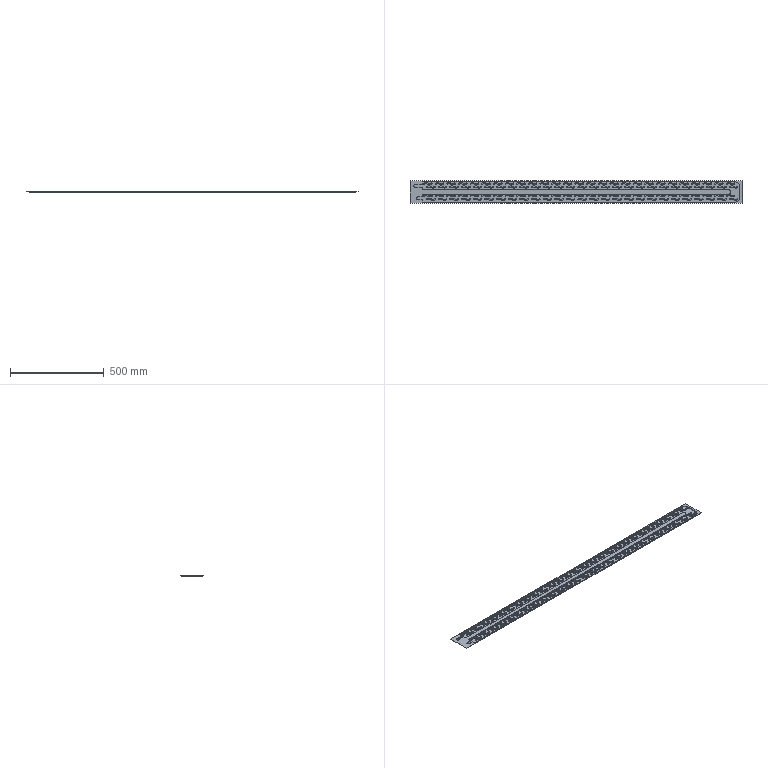Part | SolidWorks | features ICE 7, LPattern 2, BaseBody 1 | 1 solid | 1776 faces | box 1768 x 120 x 5 mm | volume 283720 mm3 | cylinder 1524 | plane 252 | commonest cylinder face diameters 4 x324 6 x324 29 x216 31 x216 39 x216 41 x216